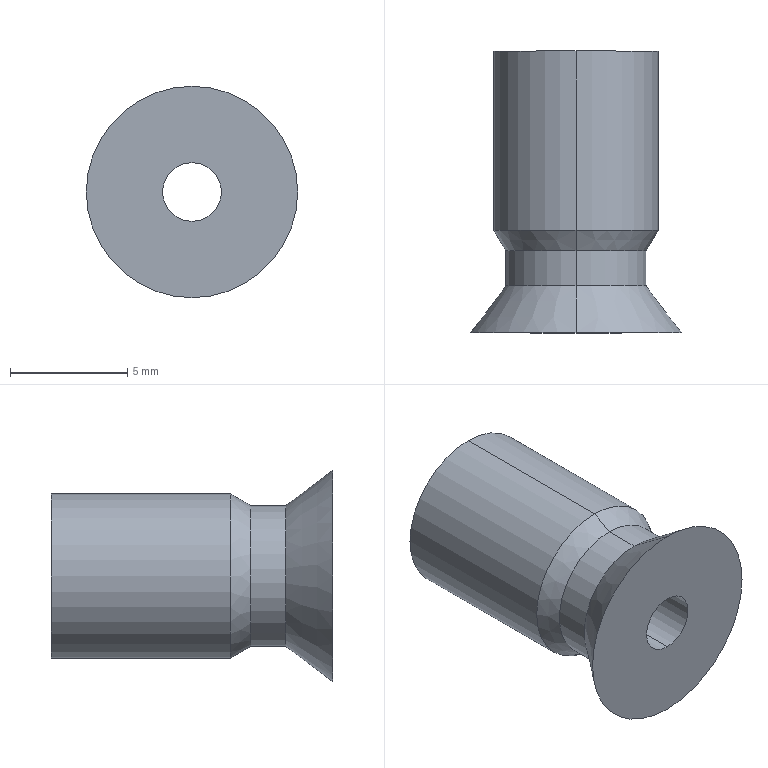Part | SolidWorks | features RefAxis 6, 3DProfileFeature 2, Revolution 1 | 1 solid | 12 faces | box 9 x 12 x 9 mm | volume 395.605 mm3 | cylinder 6 | cone 4 | plane 2 | commonest cylinder face diameters 2.5 x2 6 x2 7 x2
STEP:
#1=CARTESIAN_POINT('',(0.,4.37,3.5));
#2=VERTEX_POINT('',#1);
#3=CARTESIAN_POINT('',(0.,4.37,-3.5));
#4=VERTEX_POINT('',#3);
#5=CARTESIAN_POINT('',(0.,4.37,0.));
#6=DIRECTION('',(0.,1.,0.));
#7=DIRECTION('',(0.,0.,1.));
#8=AXIS2_PLACEMENT_3D('',#5,#6,#7);
#9=CIRCLE('',#8,3.5);
#10=EDGE_CURVE('',#2,#4,#9,.T.);
#11=ORIENTED_EDGE('',*,*,#10,.T.);
#12=CARTESIAN_POINT('',(0.,12.,-3.5));
#13=VERTEX_POINT('',#12);
#14=CARTESIAN_POINT('',(0.,0.,-3.5));
#15=DIRECTION('',(0.,1.,0.));
#16=VECTOR('',#15,1000.);
#17=LINE('',#14,#16);
#18=EDGE_CURVE('',#4,#13,#17,.T.);
#19=ORIENTED_EDGE('',*,*,#18,.T.);
#20=CARTESIAN_POINT('',(0.,12.,3.5));
#21=VERTEX_POINT('',#20);
#22=CARTESIAN_POINT('',(0.,12.,0.));
#23=DIRECTION('',(0.,1.,0.));
#24=DIRECTION('',(0.,0.,1.));
#25=AXIS2_PLACEMENT_3D('',#22,#23,#24);
#26=CIRCLE('',#25,3.5);
#27=EDGE_CURVE('',#21,#13,#26,.T.);
#28=ORIENTED_EDGE('',*,*,#27,.F.);
#29=CARTESIAN_POINT('',(0.,0.,3.5));
#30=DIRECTION('',(0.,1.,0.));
#31=VECTOR('',#30,1000.);
#32=LINE('',#29,#31);
#33=EDGE_CURVE('',#2,#21,#32,.T.);
#34=ORIENTED_EDGE('',*,*,#33,.F.);
#35=EDGE_LOOP('',(#11,#19,#28,#34));
#36=FACE_OUTER_BOUND('',#35,.T.);
#37=CARTESIAN_POINT('',(0.,0.,0.));
#38=DIRECTION('',(0.,1.,0.));
#39=DIRECTION('',(0.,0.,1.));
#40=AXIS2_PLACEMENT_3D('',#37,#38,#39);
#41=CYLINDRICAL_SURFACE('',#40,3.5);
#42=ADVANCED_FACE('',(#36),#41,.T.);
#43=CARTESIAN_POINT('',(0.,3.5,3.));
#44=VERTEX_POINT('',#43);
#45=CARTESIAN_POINT('',(0.,3.5,-3.));
#46=VERTEX_POINT('',#45);
#47=CARTESIAN_POINT('',(0.,3.5,0.));
#48=DIRECTION('',(0.,1.,0.));
#49=DIRECTION('',(0.,0.,1.));
#50=AXIS2_PLACEMENT_3D('',#47,#48,#49);
#51=CIRCLE('',#50,3.);
#52=EDGE_CURVE('',#44,#46,#51,.T.);
#53=ORIENTED_EDGE('',*,*,#52,.T.);
#54=CARTESIAN_POINT('',(0.,3.5,-3.));
#55=DIRECTION('',(0.,0.867,-0.4983));
#56=VECTOR('',#55,1000.);
#57=LINE('',#54,#56);
#58=EDGE_CURVE('',#46,#4,#57,.T.);
#59=ORIENTED_EDGE('',*,*,#58,.T.);
#60=ORIENTED_EDGE('',*,*,#10,.F.);
#61=CARTESIAN_POINT('',(0.,3.5,3.));
#62=DIRECTION('',(0.,0.867,0.4983));
#63=VECTOR('',#62,1000.);
#64=LINE('',#61,#63);
#65=EDGE_CURVE('',#44,#2,#64,.T.);
#66=ORIENTED_EDGE('',*,*,#65,.F.);
#67=EDGE_LOOP('',(#53,#59,#60,#66));
#68=FACE_OUTER_BOUND('',#67,.T.);
#69=CARTESIAN_POINT('',(0.,3.5,0.));
#70=DIRECTION('',(0.,1.,0.));
#71=DIRECTION('',(0.,0.,1.));
#72=AXIS2_PLACEMENT_3D('',#69,#70,#71);
#73=CONICAL_SURFACE('',#72,3.,0.5216);
#74=ADVANCED_FACE('',(#68),#73,.T.);
#75=CARTESIAN_POINT('',(0.,2.,3.));
#76=VERTEX_POINT('',#75);
#77=CARTESIAN_POINT('',(0.,2.,-3.));
#78=VERTEX_POINT('',#77);
#79=CARTESIAN_POINT('',(0.,2.,0.));
#80=DIRECTION('',(0.,1.,0.));
#81=DIRECTION('',(0.,0.,1.));
#82=AXIS2_PLACEMENT_3D('',#79,#80,#81);
#83=CIRCLE('',#82,3.);
#84=EDGE_CURVE('',#76,#78,#83,.T.);
#85=ORIENTED_EDGE('',*,*,#84,.T.);
#86=CARTESIAN_POINT('',(0.,0.,-3.));
#87=DIRECTION('',(0.,1.,0.));
#88=VECTOR('',#87,1000.);
#89=LINE('',#86,#88);
#90=EDGE_CURVE('',#78,#46,#89,.T.);
#91=ORIENTED_EDGE('',*,*,#90,.T.);
#92=ORIENTED_EDGE('',*,*,#52,.F.);
#93=CARTESIAN_POINT('',(0.,0.,3.));
#94=DIRECTION('',(0.,1.,0.));
#95=VECTOR('',#94,1000.);
#96=LINE('',#93,#95);
#97=EDGE_CURVE('',#76,#44,#96,.T.);
#98=ORIENTED_EDGE('',*,*,#97,.F.);
#99=EDGE_LOOP('',(#85,#91,#92,#98));
#100=FACE_OUTER_BOUND('',#99,.T.);
#101=CARTESIAN_POINT('',(0.,0.,0.));
#102=DIRECTION('',(0.,1.,0.));
#103=DIRECTION('',(0.,0.,1.));
#104=AXIS2_PLACEMENT_3D('',#101,#102,#103);
#105=CYLINDRICAL_SURFACE('',#104,3.);
#106=ADVANCED_FACE('',(#100),#105,.T.);
#107=ORIENTED_EDGE('',*,*,#84,.F.);
#108=CARTESIAN_POINT('',(0.,0.,4.5));
#109=VERTEX_POINT('',#108);
#110=CARTESIAN_POINT('',(0.,0.,4.5));
#111=DIRECTION('',(0.,-0.8,0.6));
#112=VECTOR('',#111,1000.);
#113=LINE('',#110,#112);
#114=EDGE_CURVE('',#76,#109,#113,.T.);
#115=ORIENTED_EDGE('',*,*,#114,.T.);
#116=CARTESIAN_POINT('',(0.,0.,-4.5));
#117=VERTEX_POINT('',#116);
#118=CARTESIAN_POINT('',(0.,0.,0.));
#119=DIRECTION('',(0.,1.,0.));
#120=DIRECTION('',(0.,0.,1.));
#121=AXIS2_PLACEMENT_3D('',#118,#119,#120);
#122=CIRCLE('',#121,4.5);
#123=EDGE_CURVE('',#109,#117,#122,.T.);
#124=ORIENTED_EDGE('',*,*,#123,.T.);
#125=CARTESIAN_POINT('',(0.,0.,-4.5));
#126=DIRECTION('',(0.,-0.8,-0.6));
#127=VECTOR('',#126,1000.);
#128=LINE('',#125,#127);
#129=EDGE_CURVE('',#78,#117,#128,.T.);
#130=ORIENTED_EDGE('',*,*,#129,.F.);
#131=EDGE_LOOP('',(#107,#115,#124,#130));
#132=FACE_OUTER_BOUND('',#131,.T.);
#133=CARTESIAN_POINT('',(0.,0.,0.));
#134=DIRECTION('',(0.,-1.,0.));
#135=DIRECTION('',(0.,0.,-1.));
#136=AXIS2_PLACEMENT_3D('',#133,#134,#135);
#137=CONICAL_SURFACE('',#136,4.5,0.6435);
#138=ADVANCED_FACE('',(#132),#137,.T.);
#139=CARTESIAN_POINT('',(0.,0.,-1.25));
#140=VERTEX_POINT('',#139);
#141=CARTESIAN_POINT('',(0.,0.,1.25));
#142=VERTEX_POINT('',#141);
#143=CARTESIAN_POINT('',(0.,0.,0.));
#144=DIRECTION('',(0.,1.,0.));
#145=DIRECTION('',(0.,0.,1.));
#146=AXIS2_PLACEMENT_3D('',#143,#144,#145);
#147=CIRCLE('',#146,1.25);
#148=EDGE_CURVE('',#140,#142,#147,.T.);
#149=ORIENTED_EDGE('',*,*,#148,.F.);
#150=CARTESIAN_POINT('',(0.,12.,-1.25));
#151=VERTEX_POINT('',#150);
#152=CARTESIAN_POINT('',(0.,0.,-1.25));
#153=DIRECTION('',(0.,1.,0.));
#154=VECTOR('',#153,1000.);
#155=LINE('',#152,#154);
#156=EDGE_CURVE('',#140,#151,#155,.T.);
#157=ORIENTED_EDGE('',*,*,#156,.T.);
#158=CARTESIAN_POINT('',(0.,12.,1.25));
#159=VERTEX_POINT('',#158);
#160=CARTESIAN_POINT('',(0.,12.,0.));
#161=DIRECTION('',(0.,1.,0.));
#162=DIRECTION('',(0.,0.,1.));
#163=AXIS2_PLACEMENT_3D('',#160,#161,#162);
#164=CIRCLE('',#163,1.25);
#165=EDGE_CURVE('',#151,#159,#164,.T.);
#166=ORIENTED_EDGE('',*,*,#165,.T.);
#167=CARTESIAN_POINT('',(0.,0.,1.25));
#168=DIRECTION('',(0.,1.,0.));
#169=VECTOR('',#168,1000.);
#170=LINE('',#167,#169);
#171=EDGE_CURVE('',#142,#159,#170,.T.);
#172=ORIENTED_EDGE('',*,*,#171,.F.);
#173=EDGE_LOOP('',(#149,#157,#166,#172));
#174=FACE_OUTER_BOUND('',#173,.T.);
#175=CARTESIAN_POINT('',(0.,0.,0.));
#176=DIRECTION('',(0.,1.,0.));
#177=DIRECTION('',(0.,0.,1.));
#178=AXIS2_PLACEMENT_3D('',#175,#176,#177);
#179=CYLINDRICAL_SURFACE('',#178,1.25);
#180=ADVANCED_FACE('',(#174),#179,.F.);
#181=ORIENTED_EDGE('',*,*,#156,.F.);
#182=CARTESIAN_POINT('',(0.,0.,0.));
#183=DIRECTION('',(0.,1.,0.));
#184=DIRECTION('',(0.,0.,1.));
#185=AXIS2_PLACEMENT_3D('',#182,#183,#184);
#186=CIRCLE('',#185,1.25);
#187=EDGE_CURVE('',#142,#140,#186,.T.);
#188=ORIENTED_EDGE('',*,*,#187,.F.);
#189=ORIENTED_EDGE('',*,*,#171,.T.);
#190=CARTESIAN_POINT('',(0.,12.,0.));
#191=DIRECTION('',(0.,1.,0.));
#192=DIRECTION('',(0.,0.,1.));
#193=AXIS2_PLACEMENT_3D('',#190,#191,#192);
#194=CIRCLE('',#193,1.25);
#195=EDGE_CURVE('',#159,#151,#194,.T.);
#196=ORIENTED_EDGE('',*,*,#195,.T.);
#197=EDGE_LOOP('',(#181,#188,#189,#196));
#198=FACE_OUTER_BOUND('',#197,.T.);
#199=CARTESIAN_POINT('',(0.,0.,0.));
#200=DIRECTION('',(0.,1.,0.));
#201=DIRECTION('',(0.,0.,1.));
#202=AXIS2_PLACEMENT_3D('',#199,#200,#201);
#203=CYLINDRICAL_SURFACE('',#202,1.25);
#204=ADVANCED_FACE('',(#198),#203,.F.);
#205=CARTESIAN_POINT('',(0.,0.,0.));
#206=DIRECTION('',(0.,1.,0.));
#207=DIRECTION('',(0.,0.,1.));
#208=AXIS2_PLACEMENT_3D('',#205,#206,#207);
#209=CIRCLE('',#208,4.5);
#210=EDGE_CURVE('',#117,#109,#209,.T.);
#211=ORIENTED_EDGE('',*,*,#210,.F.);
#212=ORIENTED_EDGE('',*,*,#123,.F.);
#213=EDGE_LOOP('',(#211,#212));
#214=FACE_OUTER_BOUND('',#213,.T.);
#215=ORIENTED_EDGE('',*,*,#187,.T.);
#216=ORIENTED_EDGE('',*,*,#148,.T.);
#217=EDGE_LOOP('',(#215,#216));
#218=FACE_BOUND('',#217,.T.);
#219=CARTESIAN_POINT('',(1.25,0.,0.));
#220=DIRECTION('',(0.,1.,0.));
#221=DIRECTION('',(0.,0.,1.));
#222=AXIS2_PLACEMENT_3D('',#219,#220,#221);
#223=PLANE('',#222);
#224=ADVANCED_FACE('',(#214,#218),#223,.F.);
#225=ORIENTED_EDGE('',*,*,#114,.F.);
#226=CARTESIAN_POINT('',(0.,2.,0.));
#227=DIRECTION('',(0.,1.,0.));
#228=DIRECTION('',(0.,0.,1.));
#229=AXIS2_PLACEMENT_3D('',#226,#227,#228);
#230=CIRCLE('',#229,3.);
#231=EDGE_CURVE('',#78,#76,#230,.T.);
#232=ORIENTED_EDGE('',*,*,#231,.F.);
#233=ORIENTED_EDGE('',*,*,#129,.T.);
#234=ORIENTED_EDGE('',*,*,#210,.T.);
#235=EDGE_LOOP('',(#225,#232,#233,#234));
#236=FACE_OUTER_BOUND('',#235,.T.);
#237=CARTESIAN_POINT('',(0.,0.,0.));
#238=DIRECTION('',(0.,-1.,0.));
#239=DIRECTION('',(0.,0.,-1.));
#240=AXIS2_PLACEMENT_3D('',#237,#238,#239);
#241=CONICAL_SURFACE('',#240,4.5,0.6435);
#242=ADVANCED_FACE('',(#236),#241,.T.);
#243=ORIENTED_EDGE('',*,*,#90,.F.);
#244=ORIENTED_EDGE('',*,*,#231,.T.);
#245=ORIENTED_EDGE('',*,*,#97,.T.);
#246=CARTESIAN_POINT('',(0.,3.5,0.));
#247=DIRECTION('',(0.,1.,0.));
#248=DIRECTION('',(0.,0.,1.));
#249=AXIS2_PLACEMENT_3D('',#246,#247,#248);
#250=CIRCLE('',#249,3.);
#251=EDGE_CURVE('',#46,#44,#250,.T.);
#252=ORIENTED_EDGE('',*,*,#251,.F.);
#253=EDGE_LOOP('',(#243,#244,#245,#252));
#254=FACE_OUTER_BOUND('',#253,.T.);
#255=CARTESIAN_POINT('',(0.,0.,0.));
#256=DIRECTION('',(0.,1.,0.));
#257=DIRECTION('',(0.,0.,1.));
#258=AXIS2_PLACEMENT_3D('',#255,#256,#257);
#259=CYLINDRICAL_SURFACE('',#258,3.);
#260=ADVANCED_FACE('',(#254),#259,.T.);
#261=ORIENTED_EDGE('',*,*,#58,.F.);
#262=ORIENTED_EDGE('',*,*,#251,.T.);
#263=ORIENTED_EDGE('',*,*,#65,.T.);
#264=CARTESIAN_POINT('',(0.,4.37,0.));
#265=DIRECTION('',(0.,1.,0.));
#266=DIRECTION('',(0.,0.,1.));
#267=AXIS2_PLACEMENT_3D('',#264,#265,#266);
#268=CIRCLE('',#267,3.5);
#269=EDGE_CURVE('',#4,#2,#268,.T.);
#270=ORIENTED_EDGE('',*,*,#269,.F.);
#271=EDGE_LOOP('',(#261,#262,#263,#270));
#272=FACE_OUTER_BOUND('',#271,.T.);
#273=CARTESIAN_POINT('',(0.,3.5,0.));
#274=DIRECTION('',(0.,1.,0.));
#275=DIRECTION('',(0.,0.,1.));
#276=AXIS2_PLACEMENT_3D('',#273,#274,#275);
#277=CONICAL_SURFACE('',#276,3.,0.5216);
#278=ADVANCED_FACE('',(#272),#277,.T.);
#279=ORIENTED_EDGE('',*,*,#18,.F.);
#280=ORIENTED_EDGE('',*,*,#269,.T.);
#281=ORIENTED_EDGE('',*,*,#33,.T.);
#282=CARTESIAN_POINT('',(0.,12.,0.));
#283=DIRECTION('',(0.,1.,0.));
#284=DIRECTION('',(0.,0.,1.));
#285=AXIS2_PLACEMENT_3D('',#282,#283,#284);
#286=CIRCLE('',#285,3.5);
#287=EDGE_CURVE('',#13,#21,#286,.T.);
#288=ORIENTED_EDGE('',*,*,#287,.F.);
#289=EDGE_LOOP('',(#279,#280,#281,#288));
#290=FACE_OUTER_BOUND('',#289,.T.);
#291=CARTESIAN_POINT('',(0.,0.,0.));
#292=DIRECTION('',(0.,1.,0.));
#293=DIRECTION('',(0.,0.,1.));
#294=AXIS2_PLACEMENT_3D('',#291,#292,#293);
#295=CYLINDRICAL_SURFACE('',#294,3.5);
#296=ADVANCED_FACE('',(#290),#295,.T.);
#297=ORIENTED_EDGE('',*,*,#195,.F.);
#298=ORIENTED_EDGE('',*,*,#165,.F.);
#299=EDGE_LOOP('',(#297,#298));
#300=FACE_BOUND('',#299,.T.);
#301=ORIENTED_EDGE('',*,*,#27,.T.);
#302=ORIENTED_EDGE('',*,*,#287,.T.);
#303=EDGE_LOOP('',(#301,#302));
#304=FACE_OUTER_BOUND('',#303,.T.);
#305=CARTESIAN_POINT('',(3.5,12.,0.));
#306=DIRECTION('',(0.,-1.,0.));
#307=DIRECTION('',(0.,0.,-1.));
#308=AXIS2_PLACEMENT_3D('',#305,#306,#307);
#309=PLANE('',#308);
#310=ADVANCED_FACE('',(#300,#304),#309,.F.);
#311=CLOSED_SHELL('',(#42,#74,#106,#138,#180,#204,#224,#242,#260,#278,#296,#310));
#312=MANIFOLD_SOLID_BREP('',#311);
#313=CARTESIAN_POINT('',(0.,0.,0.));
#314=DIRECTION('',(0.,0.,1.));
#315=DIRECTION('',(1.,0.,0.));
#316=AXIS2_PLACEMENT_3D('',#313,#314,#315);
#317=(LENGTH_UNIT()NAMED_UNIT(*)SI_UNIT(.MILLI.,.METRE.));
#318=UNCERTAINTY_MEASURE_WITH_UNIT(LENGTH_MEASURE(0.00001),#317,'','');
#319=(NAMED_UNIT(*)PLANE_ANGLE_UNIT()SI_UNIT($,.RADIAN.));
#320=(NAMED_UNIT(*)SI_UNIT($,.STERADIAN.)SOLID_ANGLE_UNIT());
#321=(GEOMETRIC_REPRESENTATION_CONTEXT(3)GLOBAL_UNCERTAINTY_ASSIGNED_CONTEXT((#318))GLOBAL_UNIT_ASSIGNED_CONTEXT((#317,#319,#320))REPRESENTATION_CONTEXT('',''));
#322=ADVANCED_BREP_SHAPE_REPRESENTATION('',(#312,#316),#321);